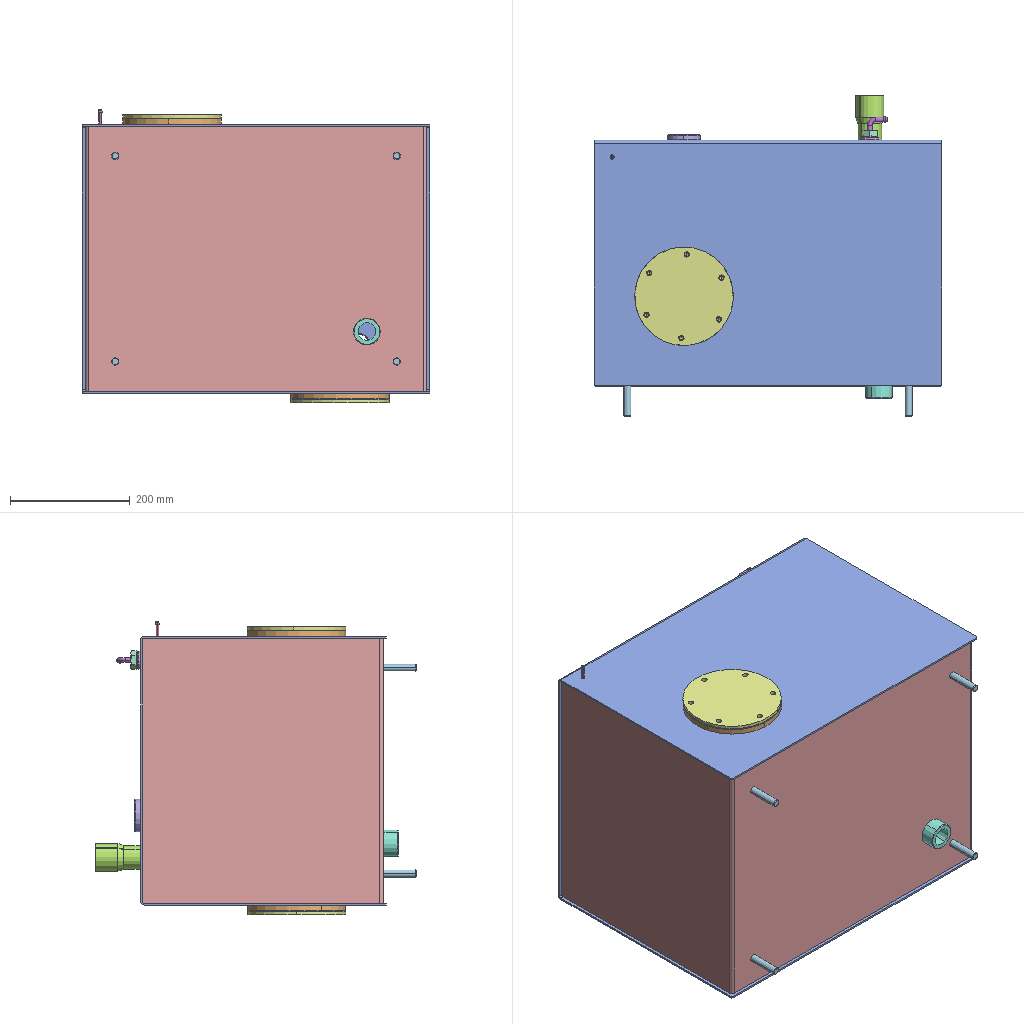Assembly | SolidWorks | 14 different items | 20 placed | box 581 x 536 x 491 mm
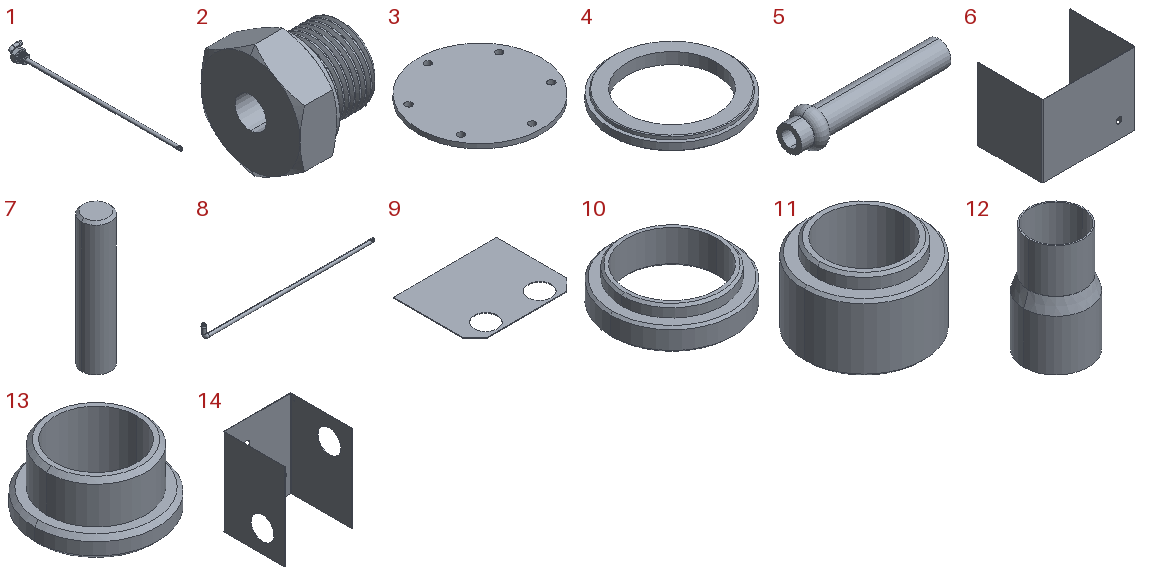Parts list (item | name | quantity | parent item | size | volume | features):
1 | (subassembly) | x1 | - | 43.501 x 435 x 31.18 mm | 19603 mm3 | features CompositeCurve 2
2 | - | x1 | in 1 | 25.4 x 27.003 x 31.18 mm | 9595 mm3 | features ICE 3, Chamfer 1, Revolution 1, SweepThread 1
3 | - | x3 | - | 165 x 165 x 6 mm | 126005 mm3 | features FlatPattern 1, SMBaseFlange 1, SheetMetal 1
4 | - | x2 | - | 165 x 165 x 15 mm | 136481 mm3 | features 3DProfileFeature 1, Chamfer 1, Extrusion 1, HoleWzd 1, ICE 1
5 | - | x1 | - | 30 x 7 x 7 mm | 414.784 mm3 | features Fillet 1, Revolution 1
6 | - | x1 | - | 571 x 403 x 444 mm | 1818117 mm3 | features ICE 2, FlatPattern 1, SMBaseFlange 1, SheetMetal 1
7 | - | x4 | - | 12 x 12 x 55 mm | 6203 mm3 | features Chamfer 1, Extrusion 1
8 | - | x1 | in 1 | 435 x 10 x 34 mm | 10005 mm3 | features ICE 2, Fillet 1, Revolution 1, Sweep 1
9 | - | x1 | - | 444 x 350 x 3 mm | 411576 mm3 | features FlatPattern 1, SMBaseFlange 1, SheetMetal 1
10 | - | x1 | - | 55 x 55 x 15 mm | 12557 mm3 | features Chamfer 1, Extrusion 1, ICE 1
11 | - | x1 | - | 45 x 45 x 30 mm | 23873 mm3 | features Chamfer 1, Extrusion 1, ICE 1
12 | - | x1 | - | 47 x 47 x 79 mm | 10172 mm3 | features 3DProfileFeature 2, ICE 2, NetBlend 1, NetBlendCut 1
13 | - | x1 | - | 30 x 30 x 15 mm | 3311 mm3 | features Chamfer 1, Extrusion 1, ICE 1
14 | - | x1 | - | 450 x 411 x 581 mm | 2075079 mm3 | features ICE 4, FlatPattern 1, SMBaseFlange 1, SheetMetal 1
Mates (type | each side: item.copy, entity, surface, feature):
In the top assembly
Coincident | 6.1 face plane Base-Flange1 | 14.1 face plane Base-Flange1 | 2 times
DistanceDim | 14.1 face plane Base-Flange1 | 6.1 face plane Base-Flange1
Concentric | 14.1 edge | 12.1 edge
DistanceDim | 12.1 face plane Boss-Extrude1 | 14.1 face plane Base-Flange1
Coincident | 14.1 face plane Base-Flange1 | 13.1 face plane Boss-Extrude1
Concentric | 14.1 edge | 13.1 edge
Coincident | 14.1 face plane Base-Flange1 | 4.1 face plane Boss-Extrude1
Concentric | 14.1 edge | 4.1 edge
Coincident | 14.1 face plane Base-Flange1 | 4.2 face plane Boss-Extrude1
Concentric | 14.1 edge | 4.2 edge
Coincident | 6.1 face plane Base-Flange1 | 11.1 face plane Boss-Extrude1
Concentric | 6.1 edge | 11.1 edge
Coincident | 14.1 face plane Base-Flange1 | 10.1 face plane Cut-Extrude1
Concentric | 14.1 edge | 10.1 edge
Coincident | 6.1 face plane Base-Flange1 | 9.1 face plane Base-Flange1 | 2 times
DistanceDim | 6.1 face plane Base-Flange1 | 9.1 face plane Base-Flange1
Concentric | 14.1 face cylinder Cut-Extrude1 | 5.1 face cylinder Revolve1
DistanceDim | 5.1 face plane Revolve1 | 14.1 face plane Base-Flange1
Coincident | 6.1 face plane Base-Flange1 | 7.1 face plane Boss-Extrude1
Coincident | 6.1 face plane Base-Flange1 | 7.2 face plane Boss-Extrude1
Coincident | 6.1 face plane Base-Flange1 | 7.3 face plane Boss-Extrude1
Coincident | 6.1 face plane Base-Flange1 | 7.4 face plane Boss-Extrude1
Coincident | 4.2 face plane Boss-Extrude1 | 3.1 face plane Base-Flange1
Concentric | 4.2 face cylinder M8 Tapped Hole1 | 3.1 face cylinder Base-Flange1 | 2 times
Coincident | 4.1 face plane Boss-Extrude1 | 3.2 face plane Base-Flange1
Concentric | 4.1 face cylinder M8 Tapped Hole1 | 3.2 face cylinder Base-Flange1 | 2 times
DistanceDim | 4.1 face cylinder M8 Tapped Hole1 | 14.1 face plane Base-Flange1
Coincident | 4.1 face plane Boss-Extrude1 | 3.3 edge
Concentric | 4.1 face cylinder M8 Tapped Hole1 | 3.3 face cylinder Base-Flange1 | 2 times
Concentric | 13.1 face cylinder Boss-Extrude1 | 8.1 face cylinder Sweep1
Coincident | 13.1 face plane Boss-Extrude1 | 2.1 face plane Revolve2
In subassembly 1
Concentric | 8.2 face cylinder Sweep1 | 2.2 face cylinder Revolve2
DistanceDim | 2.2 face plane Revolve2 | 8.2 face cylinder Sweep1
Parallel | 8.2 face plane Sweep1 | 2.2 face plane Cut-Extrude1